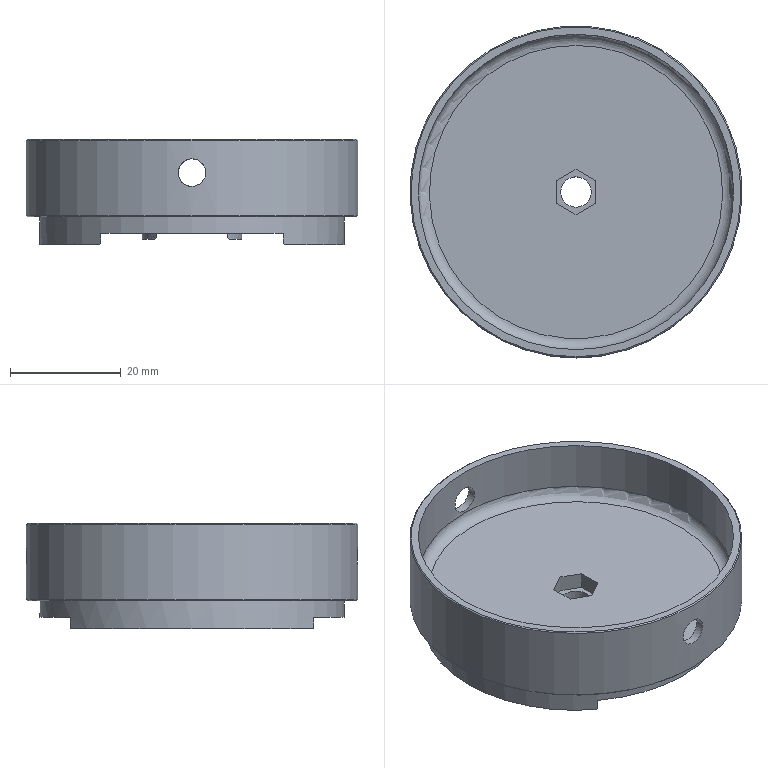CAM job | NX | 3-axis milling, drilling | part box 60 x 60 x 19 mm | stock box 74 x 74 x 60 mm
Tools:
number,name,description,diameter,corner_radius,flute_length,length,flutes
1,D63,Milling Tool-5 Parameters,63.0,0.0,50.0,75.0,2
6,D8A45,Milling Tool-5 Parameters,8.0,0.0,50.0,75.0,2
15,5.5ZT,Drilling Tool,5.5,0.0,35.0,50.0,2
19,D17R0.8,Milling Tool-5 Parameters,17.0,0.8,50.0,75.0,2
9,D10,Milling Tool-5 Parameters,10.0,0.0,50.0,75.0,2
7,D6,Milling Tool-5 Parameters,6.0,0.0,50.0,75.0,2
22,D4,Milling Tool-5 Parameters,4.0,0.0,50.0,75.0,2
23,D2,Milling Tool-5 Parameters,2.0,0.0,50.0,75.0,2
Operations:
program,operation,operation_type,tool,method,geometry_group,spindle_rpm,surface_speed,feed_per_tooth,feed_cut,feed_plunge,cut_length_mm,path_length_mm,cut_time_min,machine_time_min
1,FLOOR_WALL,VolumeBased25DMillingOperation,D63,METHOD,A,1200.0,237.0,0.5208,1250.0,100.0,313.838,367.838,0.2511,0.2565
1,DRILLING,Operation,D8A45,METHOD,A,5000.0,94.0,0.025,250.0,0.0,4.0,68.0,0.016,0.0224
1,DRILLING_COPY,Operation,5.5ZT,METHOD,A,1000.0,43.0,0.075,150.0,0.0,14.652,89.305,0.0977,0.1051
1,ZLEVEL_PROFILE,ZLevelMilling,D17R0.8,METHOD,A,2000.0,106.0,0.5,2000.0,1000.0,3913.072,3974.922,1.974,1.98
1,ZLEVEL_PROFILE_COPY,ZLevelMilling,D17R0.8,METHOD,A,2000.0,106.0,0.5,2000.0,1000.0,12195.459,12277.459,6.115,6.123
1,FLOOR_WALL_1,VolumeBased25DMillingOperation,D6,METHOD,A,4500.0,84.0,0.2,1800.0,1000.0,9601.575,10008.958,5.389,5.43
1,FLOOR_WALL_1_COPY,VolumeBased25DMillingOperation,D6,METHOD,A,6500.0,122.0,0.0769,1000.0,1000.0,855.067,1244.51,0.8551,0.8954
1,ZLEVEL_PROFILE_COPY_1,ZLevelMilling,D10,METHOD,A,7500.0,376.0,0.0567,850.0,1000.0,212.664,279.664,0.2494,0.2561
1,ZLEVEL_PROFILE_COPY_1_COPY,ZLevelMilling,D10,METHOD,A,7500.0,376.0,0.0567,850.0,1000.0,228.379,323.379,0.2679,0.2774
1,PLANAR_MILL,PlanarMilling,D8A45,METHOD,A,7500.0,188.0,0.0833,1250.0,100.0,222.528,365.928,0.178,0.1924
1,PLANAR_MILL_COPY,PlanarMilling,D8A45,METHOD,A,7500.0,188.0,0.0833,1250.0,100.0,76.124,202.125,0.0609,0.0735
1,DRILLING_COPY_1,Operation,D8A45,METHOD,A,5000.0,94.0,0.025,250.0,0.0,6.0,76.0,0.024,0.031
1,PLANAR_MILL_COPY_COPY,PlanarMilling,D8A45,METHOD,A,7500.0,188.0,0.0833,1250.0,100.0,211.041,280.041,0.1688,0.1757
2,FLOOR_WALL_COPY,VolumeBased25DMillingOperation,D63,METHOD,B,1250.0,247.0,0.88,2200.0,100.0,7506.898,10558.335,3.412,3.717
2,FLOOR_WALL_COPY_1,VolumeBased25DMillingOperation,D63,METHOD,B,1200.0,237.0,0.5208,1250.0,100.0,441.582,495.582,0.3533,0.3587
2,FLOOR_WALL_1_COPY_1,VolumeBased25DMillingOperation,D17R0.8,METHOD,B,2000.0,106.0,0.5,2000.0,1000.0,25562.747,28150.28,14.834,15.093
2,ZLEVEL_PROFILE_COPY_COPY,ZLevelMilling,D10,METHOD,B,7500.0,376.0,0.0567,850.0,1000.0,156.43,231.43,0.1833,0.1908
2,FLOOR_WALL_1_COPY_COPY,VolumeBased25DMillingOperation,D10,METHOD,B,6500.0,122.0,0.0769,1000.0,1000.0,495.32,574.32,0.4953,0.5032
2,ZLEVEL_PROFILE_COPY_1_COPY_COPY,ZLevelMilling,D6,METHOD,B,7500.0,376.0,0.1667,2500.0,1000.0,5020.95,5098.001,2.026,2.033
2,ZLEVEL_PROFILE_COPY_1_COPY_COPY_COPY,ZLevelMilling,D4,METHOD,B,5000.0,62.0,0.165,1650.0,1000.0,441.786,523.986,0.2789,0.2871
2,ZLEVEL_PROFILE_COPY_1_COPY_COPY_COPY_COPY,ZLevelMilling,D2,METHOD,B,5000.0,31.0,0.1,1000.0,1000.0,3437.274,6001.096,3.437,3.694
2,PLANAR_MILL_COPY_1,PlanarMilling,D8A45,METHOD,B,7500.0,188.0,0.0833,1250.0,100.0,383.755,556.281,0.307,0.3243
2,PLANAR_MILL_COPY_1_COPY,PlanarMilling,D8A45,METHOD,B,7500.0,188.0,0.0833,1250.0,100.0,23.683,102.683,0.0189,0.0268